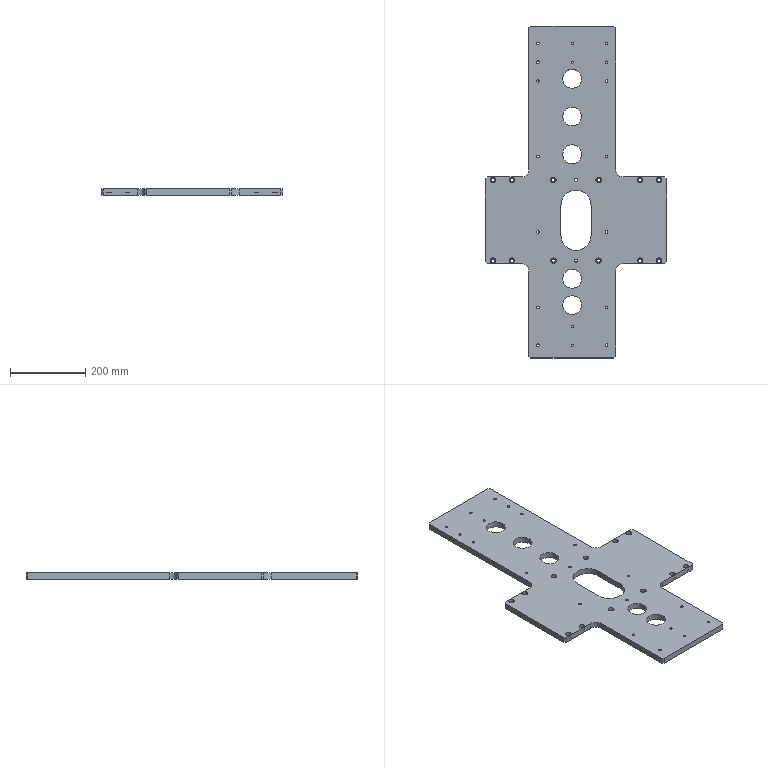Part | SolidWorks | features HoleWzd 4, Chamfer 1, Extrusion 1, Fillet 1, ICE 1 | 1 solid | 140 faces | box 480 x 880 x 16 mm | volume 3786407 mm3 | cylinder 104 | plane 36 | commonest cylinder face diameters 6.8 x28 9 x24 15 x24 50 x10 6 x8 8 x4